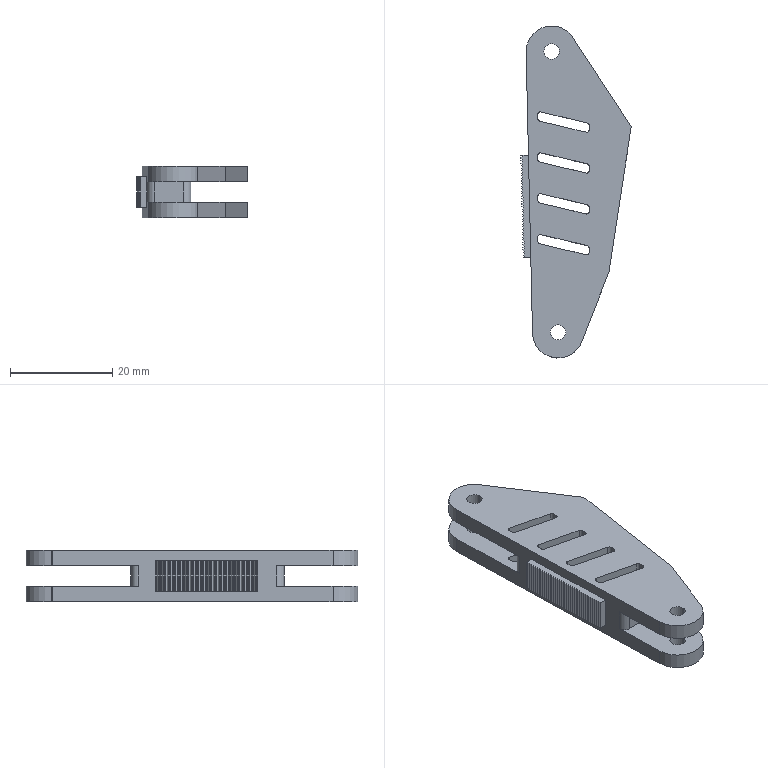Part | SolidWorks | features ICE 6, Fillet 2, Extrusion 1, LPattern 1, Scale 1 | 1 solid | 180 faces | box 21.607 x 64.987 x 10 mm | volume 6323 mm3 | plane 124 | cylinder 56 | commonest cylinder face diameters 1 x37 3 x13 10 x4 10.003 x2